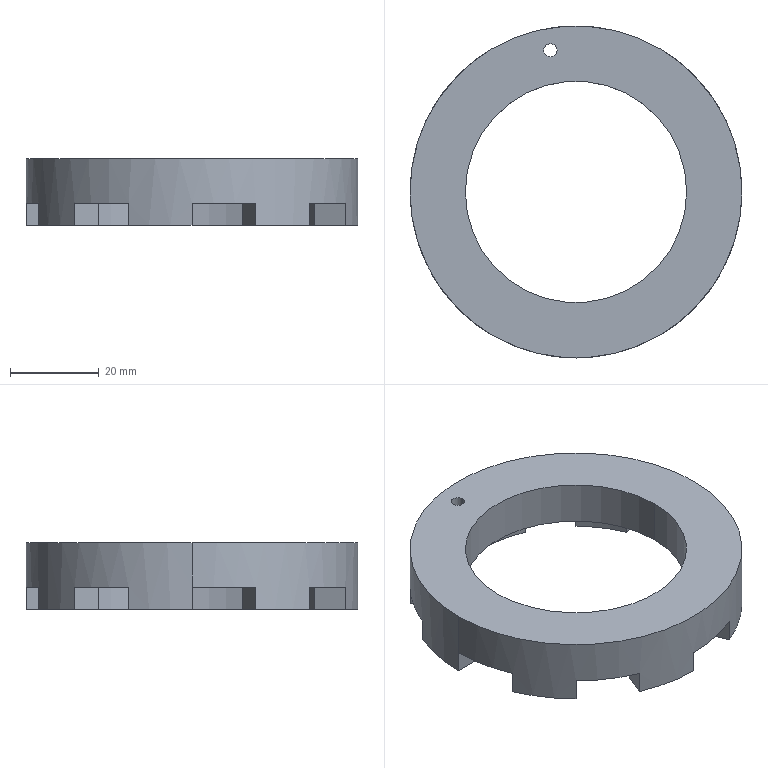Part | SolidWorks | features ICE 3, Extrusion 1 | 1 solid | 40 faces | box 75 x 75 x 15 mm | volume 28449 mm3 | plane 26 | cylinder 14 | commonest cylinder face diameters 60 x8 3 x2 50 x2 75 x2
STEP:
#1=CARTESIAN_POINT('',(-4.276,31.983,15.));
#2=VERTEX_POINT('',#1);
#3=CARTESIAN_POINT('',(-7.276,31.983,15.));
#4=VERTEX_POINT('',#3);
#5=CARTESIAN_POINT('',(-5.776,31.983,15.));
#6=DIRECTION('',(0.,0.,-1.));
#7=DIRECTION('',(-1.,0.,0.));
#8=AXIS2_PLACEMENT_3D('',#5,#6,#7);
#9=CIRCLE('',#8,1.5);
#10=EDGE_CURVE('',#2,#4,#9,.T.);
#11=ORIENTED_EDGE('',*,*,#10,.F.);
#12=CARTESIAN_POINT('',(-4.276,31.983,5.));
#13=VERTEX_POINT('',#12);
#14=CARTESIAN_POINT('',(-4.276,31.983,15.));
#15=DIRECTION('',(0.,0.,-1.));
#16=VECTOR('',#15,1000.);
#17=LINE('',#14,#16);
#18=EDGE_CURVE('',#2,#13,#17,.T.);
#19=ORIENTED_EDGE('',*,*,#18,.T.);
#20=CARTESIAN_POINT('',(-7.276,31.983,5.));
#21=VERTEX_POINT('',#20);
#22=CARTESIAN_POINT('',(-5.776,31.983,5.));
#23=DIRECTION('',(0.,0.,-1.));
#24=DIRECTION('',(-1.,0.,0.));
#25=AXIS2_PLACEMENT_3D('',#22,#23,#24);
#26=CIRCLE('',#25,1.5);
#27=EDGE_CURVE('',#13,#21,#26,.T.);
#28=ORIENTED_EDGE('',*,*,#27,.T.);
#29=CARTESIAN_POINT('',(-7.276,31.983,15.));
#30=DIRECTION('',(0.,0.,-1.));
#31=VECTOR('',#30,1000.);
#32=LINE('',#29,#31);
#33=EDGE_CURVE('',#4,#21,#32,.T.);
#34=ORIENTED_EDGE('',*,*,#33,.F.);
#35=EDGE_LOOP('',(#11,#19,#28,#34));
#36=FACE_OUTER_BOUND('',#35,.T.);
#37=CARTESIAN_POINT('',(-5.776,31.983,15.));
#38=DIRECTION('',(0.,0.,-1.));
#39=DIRECTION('',(-1.,0.,0.));
#40=AXIS2_PLACEMENT_3D('',#37,#38,#39);
#41=CYLINDRICAL_SURFACE('',#40,1.5);
#42=ADVANCED_FACE('',(#36),#41,.F.);
#43=CARTESIAN_POINT('',(37.5,0.,15.));
#44=VERTEX_POINT('',#43);
#45=CARTESIAN_POINT('',(-37.5,0.,15.));
#46=VERTEX_POINT('',#45);
#47=CARTESIAN_POINT('',(0.,0.,15.));
#48=DIRECTION('',(0.,0.,1.));
#49=DIRECTION('',(1.,0.,0.));
#50=AXIS2_PLACEMENT_3D('',#47,#48,#49);
#51=CIRCLE('',#50,37.5);
#52=EDGE_CURVE('',#44,#46,#51,.T.);
#53=ORIENTED_EDGE('',*,*,#52,.F.);
#54=CARTESIAN_POINT('',(37.5,0.,5.));
#55=VERTEX_POINT('',#54);
#56=CARTESIAN_POINT('',(37.5,0.,15.));
#57=DIRECTION('',(0.,0.,-1.));
#58=VECTOR('',#57,1000.);
#59=LINE('',#56,#58);
#60=EDGE_CURVE('',#44,#55,#59,.T.);
#61=ORIENTED_EDGE('',*,*,#60,.T.);
#62=CARTESIAN_POINT('',(34.645,14.351,5.));
#63=VERTEX_POINT('',#62);
#64=CARTESIAN_POINT('',(0.,0.,5.));
#65=DIRECTION('',(0.,0.,-1.));
#66=DIRECTION('',(-1.,0.,0.));
#67=AXIS2_PLACEMENT_3D('',#64,#65,#66);
#68=CIRCLE('',#67,37.5);
#69=EDGE_CURVE('',#63,#55,#68,.T.);
#70=ORIENTED_EDGE('',*,*,#69,.F.);
#71=CARTESIAN_POINT('',(34.645,14.351,0.));
#72=VERTEX_POINT('',#71);
#73=CARTESIAN_POINT('',(34.645,14.351,5.));
#74=DIRECTION('',(0.,0.,-1.));
#75=VECTOR('',#74,1000.);
#76=LINE('',#73,#75);
#77=EDGE_CURVE('',#63,#72,#76,.T.);
#78=ORIENTED_EDGE('',*,*,#77,.T.);
#79=CARTESIAN_POINT('',(26.517,26.517,0.));
#80=VERTEX_POINT('',#79);
#81=CARTESIAN_POINT('',(0.,0.,0.));
#82=DIRECTION('',(0.,0.,1.));
#83=DIRECTION('',(1.,0.,0.));
#84=AXIS2_PLACEMENT_3D('',#81,#82,#83);
#85=CIRCLE('',#84,37.5);
#86=EDGE_CURVE('',#72,#80,#85,.T.);
#87=ORIENTED_EDGE('',*,*,#86,.T.);
#88=CARTESIAN_POINT('',(26.517,26.517,5.));
#89=VERTEX_POINT('',#88);
#90=CARTESIAN_POINT('',(26.517,26.517,5.));
#91=DIRECTION('',(0.,0.,-1.));
#92=VECTOR('',#91,1000.);
#93=LINE('',#90,#92);
#94=EDGE_CURVE('',#89,#80,#93,.T.);
#95=ORIENTED_EDGE('',*,*,#94,.F.);
#96=CARTESIAN_POINT('',(14.351,34.645,5.));
#97=VERTEX_POINT('',#96);
#98=CARTESIAN_POINT('',(0.,0.,5.));
#99=DIRECTION('',(0.,0.,-1.));
#100=DIRECTION('',(-1.,0.,0.));
#101=AXIS2_PLACEMENT_3D('',#98,#99,#100);
#102=CIRCLE('',#101,37.5);
#103=EDGE_CURVE('',#97,#89,#102,.T.);
#104=ORIENTED_EDGE('',*,*,#103,.F.);
#105=CARTESIAN_POINT('',(14.351,34.645,0.));
#106=VERTEX_POINT('',#105);
#107=CARTESIAN_POINT('',(14.351,34.645,5.));
#108=DIRECTION('',(0.,0.,-1.));
#109=VECTOR('',#108,1000.);
#110=LINE('',#107,#109);
#111=EDGE_CURVE('',#97,#106,#110,.T.);
#112=ORIENTED_EDGE('',*,*,#111,.T.);
#113=CARTESIAN_POINT('',(0.,37.5,0.));
#114=VERTEX_POINT('',#113);
#115=CARTESIAN_POINT('',(0.,0.,0.));
#116=DIRECTION('',(0.,0.,1.));
#117=DIRECTION('',(1.,0.,0.));
#118=AXIS2_PLACEMENT_3D('',#115,#116,#117);
#119=CIRCLE('',#118,37.5);
#120=EDGE_CURVE('',#106,#114,#119,.T.);
#121=ORIENTED_EDGE('',*,*,#120,.T.);
#122=CARTESIAN_POINT('',(0.,37.5,5.));
#123=VERTEX_POINT('',#122);
#124=CARTESIAN_POINT('',(0.,37.5,5.));
#125=DIRECTION('',(0.,0.,-1.));
#126=VECTOR('',#125,1000.);
#127=LINE('',#124,#126);
#128=EDGE_CURVE('',#123,#114,#127,.T.);
#129=ORIENTED_EDGE('',*,*,#128,.F.);
#130=CARTESIAN_POINT('',(-14.351,34.645,5.));
#131=VERTEX_POINT('',#130);
#132=CARTESIAN_POINT('',(0.,0.,5.));
#133=DIRECTION('',(0.,0.,-1.));
#134=DIRECTION('',(-1.,0.,0.));
#135=AXIS2_PLACEMENT_3D('',#132,#133,#134);
#136=CIRCLE('',#135,37.5);
#137=EDGE_CURVE('',#131,#123,#136,.T.);
#138=ORIENTED_EDGE('',*,*,#137,.F.);
#139=CARTESIAN_POINT('',(-14.351,34.645,0.));
#140=VERTEX_POINT('',#139);
#141=CARTESIAN_POINT('',(-14.351,34.645,5.));
#142=DIRECTION('',(0.,0.,-1.));
#143=VECTOR('',#142,1000.);
#144=LINE('',#141,#143);
#145=EDGE_CURVE('',#131,#140,#144,.T.);
#146=ORIENTED_EDGE('',*,*,#145,.T.);
#147=CARTESIAN_POINT('',(-26.517,26.517,0.));
#148=VERTEX_POINT('',#147);
#149=CARTESIAN_POINT('',(0.,0.,0.));
#150=DIRECTION('',(0.,0.,1.));
#151=DIRECTION('',(1.,0.,0.));
#152=AXIS2_PLACEMENT_3D('',#149,#150,#151);
#153=CIRCLE('',#152,37.5);
#154=EDGE_CURVE('',#140,#148,#153,.T.);
#155=ORIENTED_EDGE('',*,*,#154,.T.);
#156=CARTESIAN_POINT('',(-26.517,26.517,5.));
#157=VERTEX_POINT('',#156);
#158=CARTESIAN_POINT('',(-26.517,26.517,5.));
#159=DIRECTION('',(0.,0.,-1.));
#160=VECTOR('',#159,1000.);
#161=LINE('',#158,#160);
#162=EDGE_CURVE('',#157,#148,#161,.T.);
#163=ORIENTED_EDGE('',*,*,#162,.F.);
#164=CARTESIAN_POINT('',(-34.645,14.351,5.));
#165=VERTEX_POINT('',#164);
#166=CARTESIAN_POINT('',(0.,0.,5.));
#167=DIRECTION('',(0.,0.,-1.));
#168=DIRECTION('',(-1.,0.,0.));
#169=AXIS2_PLACEMENT_3D('',#166,#167,#168);
#170=CIRCLE('',#169,37.5);
#171=EDGE_CURVE('',#165,#157,#170,.T.);
#172=ORIENTED_EDGE('',*,*,#171,.F.);
#173=CARTESIAN_POINT('',(-34.645,14.351,0.));
#174=VERTEX_POINT('',#173);
#175=CARTESIAN_POINT('',(-34.645,14.351,5.));
#176=DIRECTION('',(0.,0.,-1.));
#177=VECTOR('',#176,1000.);
#178=LINE('',#175,#177);
#179=EDGE_CURVE('',#165,#174,#178,.T.);
#180=ORIENTED_EDGE('',*,*,#179,.T.);
#181=CARTESIAN_POINT('',(-37.5,0.,0.));
#182=VERTEX_POINT('',#181);
#183=CARTESIAN_POINT('',(0.,0.,0.));
#184=DIRECTION('',(0.,0.,1.));
#185=DIRECTION('',(1.,0.,0.));
#186=AXIS2_PLACEMENT_3D('',#183,#184,#185);
#187=CIRCLE('',#186,37.5);
#188=EDGE_CURVE('',#174,#182,#187,.T.);
#189=ORIENTED_EDGE('',*,*,#188,.T.);
#190=CARTESIAN_POINT('',(-37.5,0.,5.));
#191=VERTEX_POINT('',#190);
#192=CARTESIAN_POINT('',(-37.5,0.,5.));
#193=DIRECTION('',(0.,0.,-1.));
#194=VECTOR('',#193,1000.);
#195=LINE('',#192,#194);
#196=EDGE_CURVE('',#191,#182,#195,.T.);
#197=ORIENTED_EDGE('',*,*,#196,.F.);
#198=CARTESIAN_POINT('',(-37.5,0.,15.));
#199=DIRECTION('',(0.,0.,-1.));
#200=VECTOR('',#199,1000.);
#201=LINE('',#198,#200);
#202=EDGE_CURVE('',#46,#191,#201,.T.);
#203=ORIENTED_EDGE('',*,*,#202,.F.);
#204=EDGE_LOOP('',(#53,#61,#70,#78,#87,#95,#104,#112,#121,#129,#138,#146,#155,#163,#172,#180,#189,#197,#203));
#205=FACE_OUTER_BOUND('',#204,.T.);
#206=CARTESIAN_POINT('',(0.,0.,15.));
#207=DIRECTION('',(0.,0.,-1.));
#208=DIRECTION('',(-1.,0.,0.));
#209=AXIS2_PLACEMENT_3D('',#206,#207,#208);
#210=CYLINDRICAL_SURFACE('',#209,37.5);
#211=ADVANCED_FACE('',(#205),#210,.T.);
#212=CARTESIAN_POINT('',(-25.,0.,15.));
#213=VERTEX_POINT('',#212);
#214=CARTESIAN_POINT('',(25.,0.,15.));
#215=VERTEX_POINT('',#214);
#216=CARTESIAN_POINT('',(0.,0.,15.));
#217=DIRECTION('',(0.,0.,1.));
#218=DIRECTION('',(1.,0.,0.));
#219=AXIS2_PLACEMENT_3D('',#216,#217,#218);
#220=CIRCLE('',#219,25.);
#221=EDGE_CURVE('',#213,#215,#220,.T.);
#222=ORIENTED_EDGE('',*,*,#221,.T.);
#223=CARTESIAN_POINT('',(25.,0.,5.));
#224=VERTEX_POINT('',#223);
#225=CARTESIAN_POINT('',(25.,0.,15.));
#226=DIRECTION('',(0.,0.,-1.));
#227=VECTOR('',#226,1000.);
#228=LINE('',#225,#227);
#229=EDGE_CURVE('',#215,#224,#228,.T.);
#230=ORIENTED_EDGE('',*,*,#229,.T.);
#231=CARTESIAN_POINT('',(-25.,0.,5.));
#232=VERTEX_POINT('',#231);
#233=CARTESIAN_POINT('',(0.,0.,5.));
#234=DIRECTION('',(0.,0.,-1.));
#235=DIRECTION('',(-1.,0.,0.));
#236=AXIS2_PLACEMENT_3D('',#233,#234,#235);
#237=CIRCLE('',#236,25.);
#238=EDGE_CURVE('',#224,#232,#237,.T.);
#239=ORIENTED_EDGE('',*,*,#238,.T.);
#240=CARTESIAN_POINT('',(-25.,0.,15.));
#241=DIRECTION('',(0.,0.,-1.));
#242=VECTOR('',#241,1000.);
#243=LINE('',#240,#242);
#244=EDGE_CURVE('',#213,#232,#243,.T.);
#245=ORIENTED_EDGE('',*,*,#244,.F.);
#246=EDGE_LOOP('',(#222,#230,#239,#245));
#247=FACE_OUTER_BOUND('',#246,.T.);
#248=CARTESIAN_POINT('',(0.,0.,15.));
#249=DIRECTION('',(0.,0.,-1.));
#250=DIRECTION('',(-1.,0.,0.));
#251=AXIS2_PLACEMENT_3D('',#248,#249,#250);
#252=CYLINDRICAL_SURFACE('',#251,25.);
#253=ADVANCED_FACE('',(#247),#252,.F.);
#254=CARTESIAN_POINT('',(-14.351,-34.645,0.));
#255=VERTEX_POINT('',#254);
#256=CARTESIAN_POINT('',(0.,-37.5,0.));
#257=VERTEX_POINT('',#256);
#258=CARTESIAN_POINT('',(0.,0.,0.));
#259=DIRECTION('',(0.,0.,1.));
#260=DIRECTION('',(1.,0.,0.));
#261=AXIS2_PLACEMENT_3D('',#258,#259,#260);
#262=CIRCLE('',#261,37.5);
#263=EDGE_CURVE('',#255,#257,#262,.T.);
#264=ORIENTED_EDGE('',*,*,#263,.F.);
#265=CARTESIAN_POINT('',(-11.481,-27.716,0.));
#266=VERTEX_POINT('',#265);
#267=CARTESIAN_POINT('',(-11.481,-27.716,0.));
#268=DIRECTION('',(-0.3827,-0.9239,0.));
#269=VECTOR('',#268,1000.);
#270=LINE('',#267,#269);
#271=EDGE_CURVE('',#266,#255,#270,.T.);
#272=ORIENTED_EDGE('',*,*,#271,.F.);
#273=CARTESIAN_POINT('',(0.,-30.,0.));
#274=VERTEX_POINT('',#273);
#275=CARTESIAN_POINT('',(0.,0.,0.));
#276=DIRECTION('',(0.,0.,-1.));
#277=DIRECTION('',(-1.,0.,0.));
#278=AXIS2_PLACEMENT_3D('',#275,#276,#277);
#279=CIRCLE('',#278,30.);
#280=EDGE_CURVE('',#274,#266,#279,.T.);
#281=ORIENTED_EDGE('',*,*,#280,.F.);
#282=CARTESIAN_POINT('',(0.,-30.,0.));
#283=DIRECTION('',(0.,1.,0.));
#284=VECTOR('',#283,1000.);
#285=LINE('',#282,#284);
#286=EDGE_CURVE('',#257,#274,#285,.T.);
#287=ORIENTED_EDGE('',*,*,#286,.F.);
#288=EDGE_LOOP('',(#264,#272,#281,#287));
#289=FACE_OUTER_BOUND('',#288,.T.);
#290=CARTESIAN_POINT('',(0.,0.,0.));
#291=DIRECTION('',(0.,0.,1.));
#292=DIRECTION('',(1.,0.,0.));
#293=AXIS2_PLACEMENT_3D('',#290,#291,#292);
#294=PLANE('',#293);
#295=ADVANCED_FACE('',(#289),#294,.F.);
#296=CARTESIAN_POINT('',(-21.213,21.213,0.));
#297=VERTEX_POINT('',#296);
#298=CARTESIAN_POINT('',(-11.481,27.716,0.));
#299=VERTEX_POINT('',#298);
#300=CARTESIAN_POINT('',(0.,0.,0.));
#301=DIRECTION('',(0.,0.,-1.));
#302=DIRECTION('',(-1.,0.,0.));
#303=AXIS2_PLACEMENT_3D('',#300,#301,#302);
#304=CIRCLE('',#303,30.);
#305=EDGE_CURVE('',#297,#299,#304,.T.);
#306=ORIENTED_EDGE('',*,*,#305,.F.);
#307=CARTESIAN_POINT('',(-21.213,21.213,0.));
#308=DIRECTION('',(0.7071,-0.7071,0.));
#309=VECTOR('',#308,1000.);
#310=LINE('',#307,#309);
#311=EDGE_CURVE('',#148,#297,#310,.T.);
#312=ORIENTED_EDGE('',*,*,#311,.F.);
#313=ORIENTED_EDGE('',*,*,#154,.F.);
#314=CARTESIAN_POINT('',(-11.481,27.716,0.));
#315=DIRECTION('',(-0.3827,0.9239,0.));
#316=VECTOR('',#315,1000.);
#317=LINE('',#314,#316);
#318=EDGE_CURVE('',#299,#140,#317,.T.);
#319=ORIENTED_EDGE('',*,*,#318,.F.);
#320=EDGE_LOOP('',(#306,#312,#313,#319));
#321=FACE_OUTER_BOUND('',#320,.T.);
#322=CARTESIAN_POINT('',(0.,0.,0.));
#323=DIRECTION('',(0.,0.,1.));
#324=DIRECTION('',(1.,0.,0.));
#325=AXIS2_PLACEMENT_3D('',#322,#323,#324);
#326=PLANE('',#325);
#327=ADVANCED_FACE('',(#321),#326,.F.);
#328=ORIENTED_EDGE('',*,*,#188,.F.);
#329=CARTESIAN_POINT('',(-27.716,11.481,0.));
#330=VERTEX_POINT('',#329);
#331=CARTESIAN_POINT('',(-27.716,11.481,0.));
#332=DIRECTION('',(-0.9239,0.3827,0.));
#333=VECTOR('',#332,1000.);
#334=LINE('',#331,#333);
#335=EDGE_CURVE('',#330,#174,#334,.T.);
#336=ORIENTED_EDGE('',*,*,#335,.F.);
#337=CARTESIAN_POINT('',(-30.,0.,0.));
#338=VERTEX_POINT('',#337);
#339=CARTESIAN_POINT('',(0.,0.,0.));
#340=DIRECTION('',(0.,0.,-1.));
#341=DIRECTION('',(-1.,0.,0.));
#342=AXIS2_PLACEMENT_3D('',#339,#340,#341);
#343=CIRCLE('',#342,30.);
#344=EDGE_CURVE('',#338,#330,#343,.T.);
#345=ORIENTED_EDGE('',*,*,#344,.F.);
#346=CARTESIAN_POINT('',(-30.,0.,0.));
#347=DIRECTION('',(1.,0.,0.));
#348=VECTOR('',#347,1000.);
#349=LINE('',#346,#348);
#350=EDGE_CURVE('',#182,#338,#349,.T.);
#351=ORIENTED_EDGE('',*,*,#350,.F.);
#352=EDGE_LOOP('',(#328,#336,#345,#351));
#353=FACE_OUTER_BOUND('',#352,.T.);
#354=CARTESIAN_POINT('',(0.,0.,0.));
#355=DIRECTION('',(0.,0.,1.));
#356=DIRECTION('',(1.,0.,0.));
#357=AXIS2_PLACEMENT_3D('',#354,#355,#356);
#358=PLANE('',#357);
#359=ADVANCED_FACE('',(#353),#358,.F.);
#360=CARTESIAN_POINT('',(14.351,-34.645,0.));
#361=VERTEX_POINT('',#360);
#362=CARTESIAN_POINT('',(26.517,-26.517,0.));
#363=VERTEX_POINT('',#362);
#364=CARTESIAN_POINT('',(0.,0.,0.));
#365=DIRECTION('',(0.,0.,1.));
#366=DIRECTION('',(1.,0.,0.));
#367=AXIS2_PLACEMENT_3D('',#364,#365,#366);
#368=CIRCLE('',#367,37.5);
#369=EDGE_CURVE('',#361,#363,#368,.T.);
#370=ORIENTED_EDGE('',*,*,#369,.F.);
#371=CARTESIAN_POINT('',(11.481,-27.716,0.));
#372=VERTEX_POINT('',#371);
#373=CARTESIAN_POINT('',(11.481,-27.716,0.));
#374=DIRECTION('',(0.3827,-0.9239,0.));
#375=VECTOR('',#374,1000.);
#376=LINE('',#373,#375);
#377=EDGE_CURVE('',#372,#361,#376,.T.);
#378=ORIENTED_EDGE('',*,*,#377,.F.);
#379=CARTESIAN_POINT('',(21.213,-21.213,0.));
#380=VERTEX_POINT('',#379);
#381=CARTESIAN_POINT('',(0.,0.,0.));
#382=DIRECTION('',(0.,0.,-1.));
#383=DIRECTION('',(-1.,0.,0.));
#384=AXIS2_PLACEMENT_3D('',#381,#382,#383);
#385=CIRCLE('',#384,30.);
#386=EDGE_CURVE('',#380,#372,#385,.T.);
#387=ORIENTED_EDGE('',*,*,#386,.F.);
#388=CARTESIAN_POINT('',(21.213,-21.213,0.));
#389=DIRECTION('',(-0.7071,0.7071,0.));
#390=VECTOR('',#389,1000.);
#391=LINE('',#388,#390);
#392=EDGE_CURVE('',#363,#380,#391,.T.);
#393=ORIENTED_EDGE('',*,*,#392,.F.);
#394=EDGE_LOOP('',(#370,#378,#387,#393));
#395=FACE_OUTER_BOUND('',#394,.T.);
#396=CARTESIAN_POINT('',(0.,0.,0.));
#397=DIRECTION('',(0.,0.,1.));
#398=DIRECTION('',(1.,0.,0.));
#399=AXIS2_PLACEMENT_3D('',#396,#397,#398);
#400=PLANE('',#399);
#401=ADVANCED_FACE('',(#395),#400,.F.);
#402=CARTESIAN_POINT('',(34.645,-14.351,0.));
#403=VERTEX_POINT('',#402);
#404=CARTESIAN_POINT('',(37.5,0.,0.));
#405=VERTEX_POINT('',#404);
#406=CARTESIAN_POINT('',(0.,0.,0.));
#407=DIRECTION('',(0.,0.,1.));
#408=DIRECTION('',(1.,0.,0.));
#409=AXIS2_PLACEMENT_3D('',#406,#407,#408);
#410=CIRCLE('',#409,37.5);
#411=EDGE_CURVE('',#403,#405,#410,.T.);
#412=ORIENTED_EDGE('',*,*,#411,.F.);
#413=CARTESIAN_POINT('',(27.716,-11.481,0.));
#414=VERTEX_POINT('',#413);
#415=CARTESIAN_POINT('',(27.716,-11.481,0.));
#416=DIRECTION('',(0.9239,-0.3827,0.));
#417=VECTOR('',#416,1000.);
#418=LINE('',#415,#417);
#419=EDGE_CURVE('',#414,#403,#418,.T.);
#420=ORIENTED_EDGE('',*,*,#419,.F.);
#421=CARTESIAN_POINT('',(30.,0.,0.));
#422=VERTEX_POINT('',#421);
#423=CARTESIAN_POINT('',(0.,0.,0.));
#424=DIRECTION('',(0.,0.,-1.));
#425=DIRECTION('',(-1.,0.,0.));
#426=AXIS2_PLACEMENT_3D('',#423,#424,#425);
#427=CIRCLE('',#426,30.);
#428=EDGE_CURVE('',#422,#414,#427,.T.);
#429=ORIENTED_EDGE('',*,*,#428,.F.);
#430=CARTESIAN_POINT('',(30.,0.,0.));
#431=DIRECTION('',(-1.,0.,0.));
#432=VECTOR('',#431,1000.);
#433=LINE('',#430,#432);
#434=EDGE_CURVE('',#405,#422,#433,.T.);
#435=ORIENTED_EDGE('',*,*,#434,.F.);
#436=EDGE_LOOP('',(#412,#420,#429,#435));
#437=FACE_OUTER_BOUND('',#436,.T.);
#438=CARTESIAN_POINT('',(0.,0.,0.));
#439=DIRECTION('',(0.,0.,1.));
#440=DIRECTION('',(1.,0.,0.));
#441=AXIS2_PLACEMENT_3D('',#438,#439,#440);
#442=PLANE('',#441);
#443=ADVANCED_FACE('',(#437),#442,.F.);
#444=ORIENTED_EDGE('',*,*,#86,.F.);
#445=CARTESIAN_POINT('',(27.716,11.481,0.));
#446=VERTEX_POINT('',#445);
#447=CARTESIAN_POINT('',(27.716,11.481,0.));
#448=DIRECTION('',(0.9239,0.3827,0.));
#449=VECTOR('',#448,1000.);
#450=LINE('',#447,#449);
#451=EDGE_CURVE('',#446,#72,#450,.T.);
#452=ORIENTED_EDGE('',*,*,#451,.F.);
#453=CARTESIAN_POINT('',(21.213,21.213,0.));
#454=VERTEX_POINT('',#453);
#455=CARTESIAN_POINT('',(0.,0.,0.));
#456=DIRECTION('',(0.,0.,-1.));
#457=DIRECTION('',(-1.,0.,0.));
#458=AXIS2_PLACEMENT_3D('',#455,#456,#457);
#459=CIRCLE('',#458,30.);
#460=EDGE_CURVE('',#454,#446,#459,.T.);
#461=ORIENTED_EDGE('',*,*,#460,.F.);
#462=CARTESIAN_POINT('',(21.213,21.213,0.));
#463=DIRECTION('',(-0.7071,-0.7071,0.));
#464=VECTOR('',#463,1000.);
#465=LINE('',#462,#464);
#466=EDGE_CURVE('',#80,#454,#465,.T.);
#467=ORIENTED_EDGE('',*,*,#466,.F.);
#468=EDGE_LOOP('',(#444,#452,#461,#467));
#469=FACE_OUTER_BOUND('',#468,.T.);
#470=CARTESIAN_POINT('',(0.,0.,0.));
#471=DIRECTION('',(0.,0.,1.));
#472=DIRECTION('',(1.,0.,0.));
#473=AXIS2_PLACEMENT_3D('',#470,#471,#472);
#474=PLANE('',#473);
#475=ADVANCED_FACE('',(#469),#474,.F.);
#476=ORIENTED_EDGE('',*,*,#120,.F.);
#477=CARTESIAN_POINT('',(11.481,27.716,0.));
#478=VERTEX_POINT('',#477);
#479=CARTESIAN_POINT('',(11.481,27.716,0.));
#480=DIRECTION('',(0.3827,0.9239,0.));
#481=VECTOR('',#480,1000.);
#482=LINE('',#479,#481);
#483=EDGE_CURVE('',#478,#106,#482,.T.);
#484=ORIENTED_EDGE('',*,*,#483,.F.);
#485=CARTESIAN_POINT('',(0.,30.,0.));
#486=VERTEX_POINT('',#485);
#487=CARTESIAN_POINT('',(0.,0.,0.));
#488=DIRECTION('',(0.,0.,-1.));
#489=DIRECTION('',(-1.,0.,0.));
#490=AXIS2_PLACEMENT_3D('',#487,#488,#489);
#491=CIRCLE('',#490,30.);
#492=EDGE_CURVE('',#486,#478,#491,.T.);
#493=ORIENTED_EDGE('',*,*,#492,.F.);
#494=CARTESIAN_POINT('',(0.,30.,0.));
#495=DIRECTION('',(0.,-1.,0.));
#496=VECTOR('',#495,1000.);
#497=LINE('',#494,#496);
#498=EDGE_CURVE('',#114,#486,#497,.T.);
#499=ORIENTED_EDGE('',*,*,#498,.F.);
#500=EDGE_LOOP('',(#476,#484,#493,#499));
#501=FACE_OUTER_BOUND('',#500,.T.);
#502=CARTESIAN_POINT('',(0.,0.,0.));
#503=DIRECTION('',(0.,0.,1.));
#504=DIRECTION('',(1.,0.,0.));
#505=AXIS2_PLACEMENT_3D('',#502,#503,#504);
#506=PLANE('',#505);
#507=ADVANCED_FACE('',(#501),#506,.F.);
#508=ORIENTED_EDGE('',*,*,#280,.T.);
#509=CARTESIAN_POINT('',(-11.481,-27.716,5.));
#510=VERTEX_POINT('',#509);
#511=CARTESIAN_POINT('',(-11.481,-27.716,5.));
#512=DIRECTION('',(0.,0.,-1.));
#513=VECTOR('',#512,1000.);
#514=LINE('',#511,#513);
#515=EDGE_CURVE('',#510,#266,#514,.T.);
#516=ORIENTED_EDGE('',*,*,#515,.F.);
#517=CARTESIAN_POINT('',(0.,-30.,5.));
#518=VERTEX_POINT('',#517);
#519=CARTESIAN_POINT('',(0.,0.,5.));
#520=DIRECTION('',(0.,0.,-1.));
#521=DIRECTION('',(-1.,0.,0.));
#522=AXIS2_PLACEMENT_3D('',#519,#520,#521);
#523=CIRCLE('',#522,30.);
#524=EDGE_CURVE('',#518,#510,#523,.T.);
#525=ORIENTED_EDGE('',*,*,#524,.F.);
#526=CARTESIAN_POINT('',(0.,-30.,5.));
#527=DIRECTION('',(0.,0.,-1.));
#528=VECTOR('',#527,1000.);
#529=LINE('',#526,#528);
#530=EDGE_CURVE('',#518,#274,#529,.T.);
#531=ORIENTED_EDGE('',*,*,#530,.T.);
#532=EDGE_LOOP('',(#508,#516,#525,#531));
#533=FACE_OUTER_BOUND('',#532,.T.);
#534=CARTESIAN_POINT('',(0.,0.,5.));
#535=DIRECTION('',(0.,0.,-1.));
#536=DIRECTION('',(-1.,0.,0.));
#537=AXIS2_PLACEMENT_3D('',#534,#535,#536);
#538=CYLINDRICAL_SURFACE('',#537,30.);
#539=ADVANCED_FACE('',(#533),#538,.F.);
#540=CARTESIAN_POINT('',(-21.213,21.213,5.));
#541=VERTEX_POINT('',#540);
#542=CARTESIAN_POINT('',(-11.481,27.716,5.));
#543=VERTEX_POINT('',#542);
#544=CARTESIAN_POINT('',(0.,0.,5.));
#545=DIRECTION('',(0.,0.,-1.));
#546=DIRECTION('',(-1.,0.,0.));
#547=AXIS2_PLACEMENT_3D('',#544,#545,#546);
#548=CIRCLE('',#547,30.);
#549=EDGE_CURVE('',#541,#543,#548,.T.);
#550=ORIENTED_EDGE('',*,*,#549,.F.);
#551=CARTESIAN_POINT('',(-21.213,21.213,5.));
#552=DIRECTION('',(0.,0.,-1.));
#553=VECTOR('',#552,1000.);
#554=LINE('',#551,#553);
#555=EDGE_CURVE('',#541,#297,#554,.T.);
#556=ORIENTED_EDGE('',*,*,#555,.T.);
#557=ORIENTED_EDGE('',*,*,#305,.T.);
#558=CARTESIAN_POINT('',(-11.481,27.716,5.));
#559=DIRECTION('',(0.,0.,-1.));
#560=VECTOR('',#559,1000.);
#561=LINE('',#558,#560);
#562=EDGE_CURVE('',#543,#299,#561,.T.);
#563=ORIENTED_EDGE('',*,*,#562,.F.);
#564=EDGE_LOOP('',(#550,#556,#557,#563));
#565=FACE_OUTER_BOUND('',#564,.T.);
#566=CARTESIAN_POINT('',(0.,0.,5.));
#567=DIRECTION('',(0.,0.,-1.));
#568=DIRECTION('',(-1.,0.,0.));
#569=AXIS2_PLACEMENT_3D('',#566,#567,#568);
#570=CYLINDRICAL_SURFACE('',#569,30.);
#571=ADVANCED_FACE('',(#565),#570,.F.);
#572=ORIENTED_EDGE('',*,*,#344,.T.);
#573=CARTESIAN_POINT('',(-27.716,11.481,5.));
#574=VERTEX_POINT('',#573);
#575=CARTESIAN_POINT('',(-27.716,11.481,5.));
#576=DIRECTION('',(0.,0.,-1.));
#577=VECTOR('',#576,1000.);
#578=LINE('',#575,#577);
#579=EDGE_CURVE('',#574,#330,#578,.T.);
#580=ORIENTED_EDGE('',*,*,#579,.F.);
#581=CARTESIAN_POINT('',(-30.,0.,5.));
#582=VERTEX_POINT('',#581);
#583=CARTESIAN_POINT('',(0.,0.,5.));
#584=DIRECTION('',(0.,0.,-1.));
#585=DIRECTION('',(-1.,0.,0.));
#586=AXIS2_PLACEMENT_3D('',#583,#584,#585);
#587=CIRCLE('',#586,30.);
#588=EDGE_CURVE('',#582,#574,#587,.T.);
#589=ORIENTED_EDGE('',*,*,#588,.F.);
#590=CARTESIAN_POINT('',(-30.,0.,5.));
#591=DIRECTION('',(0.,0.,-1.));
#592=VECTOR('',#591,1000.);
#593=LINE('',#590,#592);
#594=EDGE_CURVE('',#582,#338,#593,.T.);
#595=ORIENTED_EDGE('',*,*,#594,.T.);
#596=EDGE_LOOP('',(#572,#580,#589,#595));
#597=FACE_OUTER_BOUND('',#596,.T.);
#598=CARTESIAN_POINT('',(0.,0.,5.));
#599=DIRECTION('',(0.,0.,-1.));
#600=DIRECTION('',(-1.,0.,0.));
#601=AXIS2_PLACEMENT_3D('',#598,#599,#600);
#602=CYLINDRICAL_SURFACE('',#601,30.);
#603=ADVANCED_FACE('',(#597),#602,.F.);
#604=ORIENTED_EDGE('',*,*,#386,.T.);
#605=CARTESIAN_POINT('',(11.481,-27.716,5.));
#606=VERTEX_POINT('',#605);
#607=CARTESIAN_POINT('',(11.481,-27.716,5.));
#608=DIRECTION('',(0.,0.,-1.));
#609=VECTOR('',#608,1000.);
#610=LINE('',#607,#609);
#611=EDGE_CURVE('',#606,#372,#610,.T.);
#612=ORIENTED_EDGE('',*,*,#611,.F.);
#613=CARTESIAN_POINT('',(21.213,-21.213,5.));
#614=VERTEX_POINT('',#613);
#615=CARTESIAN_POINT('',(0.,0.,5.));
#616=DIRECTION('',(0.,0.,-1.));
#617=DIRECTION('',(-1.,0.,0.));
#618=AXIS2_PLACEMENT_3D('',#615,#616,#617);
#619=CIRCLE('',#618,30.);
#620=EDGE_CURVE('',#614,#606,#619,.T.);
#621=ORIENTED_EDGE('',*,*,#620,.F.);
#622=CARTESIAN_POINT('',(21.213,-21.213,5.));
#623=DIRECTION('',(0.,0.,-1.));
#624=VECTOR('',#623,1000.);
#625=LINE('',#622,#624);
#626=EDGE_CURVE('',#614,#380,#625,.T.);
#627=ORIENTED_EDGE('',*,*,#626,.T.);
#628=EDGE_LOOP('',(#604,#612,#621,#627));
#629=FACE_OUTER_BOUND('',#628,.T.);
#630=CARTESIAN_POINT('',(0.,0.,5.));
#631=DIRECTION('',(0.,0.,-1.));
#632=DIRECTION('',(-1.,0.,0.));
#633=AXIS2_PLACEMENT_3D('',#630,#631,#632);
#634=CYLINDRICAL_SURFACE('',#633,30.);
#635=ADVANCED_FACE('',(#629),#634,.F.);
#636=ORIENTED_EDGE('',*,*,#428,.T.);
#637=CARTESIAN_POINT('',(27.716,-11.481,5.));
#638=VERTEX_POINT('',#637);
#639=CARTESIAN_POINT('',(27.716,-11.481,5.));
#640=DIRECTION('',(0.,0.,-1.));
#641=VECTOR('',#640,1000.);
#642=LINE('',#639,#641);
#643=EDGE_CURVE('',#638,#414,#642,.T.);
#644=ORIENTED_EDGE('',*,*,#643,.F.);
#645=CARTESIAN_POINT('',(30.,0.,5.));
#646=VERTEX_POINT('',#645);
#647=CARTESIAN_POINT('',(0.,0.,5.));
#648=DIRECTION('',(0.,0.,-1.));
#649=DIRECTION('',(-1.,0.,0.));
#650=AXIS2_PLACEMENT_3D('',#647,#648,#649);
#651=CIRCLE('',#650,30.);
#652=EDGE_CURVE('',#646,#638,#651,.T.);
#653=ORIENTED_EDGE('',*,*,#652,.F.);
#654=CARTESIAN_POINT('',(30.,0.,5.));
#655=DIRECTION('',(0.,0.,-1.));
#656=VECTOR('',#655,1000.);
#657=LINE('',#654,#656);
#658=EDGE_CURVE('',#646,#422,#657,.T.);
#659=ORIENTED_EDGE('',*,*,#658,.T.);
#660=EDGE_LOOP('',(#636,#644,#653,#659));
#661=FACE_OUTER_BOUND('',#660,.T.);
#662=CARTESIAN_POINT('',(0.,0.,5.));
#663=DIRECTION('',(0.,0.,-1.));
#664=DIRECTION('',(-1.,0.,0.));
#665=AXIS2_PLACEMENT_3D('',#662,#663,#664);
#666=CYLINDRICAL_SURFACE('',#665,30.);
#667=ADVANCED_FACE('',(#661),#666,.F.);
#668=ORIENTED_EDGE('',*,*,#460,.T.);
#669=CARTESIAN_POINT('',(27.716,11.481,5.));
#670=VERTEX_POINT('',#669);
#671=CARTESIAN_POINT('',(27.716,11.481,5.));
#672=DIRECTION('',(0.,0.,-1.));
#673=VECTOR('',#672,1000.);
#674=LINE('',#671,#673);
#675=EDGE_CURVE('',#670,#446,#674,.T.);
#676=ORIENTED_EDGE('',*,*,#675,.F.);
#677=CARTESIAN_POINT('',(21.213,21.213,5.));
#678=VERTEX_POINT('',#677);
#679=CARTESIAN_POINT('',(0.,0.,5.));
#680=DIRECTION('',(0.,0.,-1.));
#681=DIRECTION('',(-1.,0.,0.));
#682=AXIS2_PLACEMENT_3D('',#679,#680,#681);
#683=CIRCLE('',#682,30.);
#684=EDGE_CURVE('',#678,#670,#683,.T.);
#685=ORIENTED_EDGE('',*,*,#684,.F.);
#686=CARTESIAN_POINT('',(21.213,21.213,5.));
#687=DIRECTION('',(0.,0.,-1.));
#688=VECTOR('',#687,1000.);
#689=LINE('',#686,#688);
#690=EDGE_CURVE('',#678,#454,#689,.T.);
#691=ORIENTED_EDGE('',*,*,#690,.T.);
#692=EDGE_LOOP('',(#668,#676,#685,#691));
#693=FACE_OUTER_BOUND('',#692,.T.);
#694=CARTESIAN_POINT('',(0.,0.,5.));
#695=DIRECTION('',(0.,0.,-1.));
#696=DIRECTION('',(-1.,0.,0.));
#697=AXIS2_PLACEMENT_3D('',#694,#695,#696);
#698=CYLINDRICAL_SURFACE('',#697,30.);
#699=ADVANCED_FACE('',(#693),#698,.F.);
#700=ORIENTED_EDGE('',*,*,#492,.T.);
#701=CARTESIAN_POINT('',(11.481,27.716,5.));
#702=VERTEX_POINT('',#701);
#703=CARTESIAN_POINT('',(11.481,27.716,5.));
#704=DIRECTION('',(0.,0.,-1.));
#705=VECTOR('',#704,1000.);
#706=LINE('',#703,#705);
#707=EDGE_CURVE('',#702,#478,#706,.T.);
#708=ORIENTED_EDGE('',*,*,#707,.F.);
#709=CARTESIAN_POINT('',(0.,30.,5.));
#710=VERTEX_POINT('',#709);
#711=CARTESIAN_POINT('',(0.,0.,5.));
#712=DIRECTION('',(0.,0.,-1.));
#713=DIRECTION('',(-1.,0.,0.));
#714=AXIS2_PLACEMENT_3D('',#711,#712,#713);
#715=CIRCLE('',#714,30.);
#716=EDGE_CURVE('',#710,#702,#715,.T.);
#717=ORIENTED_EDGE('',*,*,#716,.F.);
#718=CARTESIAN_POINT('',(0.,30.,5.));
#719=DIRECTION('',(0.,0.,-1.));
#720=VECTOR('',#719,1000.);
#721=LINE('',#718,#720);
#722=EDGE_CURVE('',#710,#486,#721,.T.);
#723=ORIENTED_EDGE('',*,*,#722,.T.);
#724=EDGE_LOOP('',(#700,#708,#717,#723));
#725=FACE_OUTER_BOUND('',#724,.T.);
#726=CARTESIAN_POINT('',(0.,0.,5.));
#727=DIRECTION('',(0.,0.,-1.));
#728=DIRECTION('',(-1.,0.,0.));
#729=AXIS2_PLACEMENT_3D('',#726,#727,#728);
#730=CYLINDRICAL_SURFACE('',#729,30.);
#731=ADVANCED_FACE('',(#725),#730,.F.);
#732=ORIENTED_EDGE('',*,*,#229,.F.);
#733=CARTESIAN_POINT('',(0.,0.,15.));
#734=DIRECTION('',(0.,0.,1.));
#735=DIRECTION('',(1.,0.,0.));
#736=AXIS2_PLACEMENT_3D('',#733,#734,#735);
#737=CIRCLE('',#736,25.);
#738=EDGE_CURVE('',#215,#213,#737,.T.);
#739=ORIENTED_EDGE('',*,*,#738,.T.);
#740=ORIENTED_EDGE('',*,*,#244,.T.);
#741=CARTESIAN_POINT('',(0.,0.,5.));
#742=DIRECTION('',(0.,0.,-1.));
#743=DIRECTION('',(-1.,0.,0.));
#744=AXIS2_PLACEMENT_3D('',#741,#742,#743);
#745=CIRCLE('',#744,25.);
#746=EDGE_CURVE('',#232,#224,#745,.T.);
#747=ORIENTED_EDGE('',*,*,#746,.T.);
#748=EDGE_LOOP('',(#732,#739,#740,#747));
#749=FACE_OUTER_BOUND('',#748,.T.);
#750=CARTESIAN_POINT('',(0.,0.,15.));
#751=DIRECTION('',(0.,0.,-1.));
#752=DIRECTION('',(-1.,0.,0.));
#753=AXIS2_PLACEMENT_3D('',#750,#751,#752);
#754=CYLINDRICAL_SURFACE('',#753,25.);
#755=ADVANCED_FACE('',(#749),#754,.F.);
#756=CARTESIAN_POINT('',(-5.776,31.983,15.));
#757=DIRECTION('',(0.,0.,-1.));
#758=DIRECTION('',(-1.,0.,0.));
#759=AXIS2_PLACEMENT_3D('',#756,#757,#758);
#760=CIRCLE('',#759,1.5);
#761=EDGE_CURVE('',#4,#2,#760,.T.);
#762=ORIENTED_EDGE('',*,*,#761,.T.);
#763=ORIENTED_EDGE('',*,*,#10,.T.);
#764=EDGE_LOOP('',(#762,#763));
#765=FACE_BOUND('',#764,.T.);
#766=CARTESIAN_POINT('',(0.,0.,15.));
#767=DIRECTION('',(0.,0.,1.));
#768=DIRECTION('',(1.,0.,0.));
#769=AXIS2_PLACEMENT_3D('',#766,#767,#768);
#770=CIRCLE('',#769,37.5);
#771=EDGE_CURVE('',#46,#44,#770,.T.);
#772=ORIENTED_EDGE('',*,*,#771,.T.);
#773=ORIENTED_EDGE('',*,*,#52,.T.);
#774=EDGE_LOOP('',(#772,#773));
#775=FACE_OUTER_BOUND('',#774,.T.);
#776=ORIENTED_EDGE('',*,*,#221,.F.);
#777=ORIENTED_EDGE('',*,*,#738,.F.);
#778=EDGE_LOOP('',(#776,#777));
#779=FACE_BOUND('',#778,.T.);
#780=CARTESIAN_POINT('',(0.,0.,15.));
#781=DIRECTION('',(0.,0.,1.));
#782=DIRECTION('',(1.,0.,0.));
#783=AXIS2_PLACEMENT_3D('',#780,#781,#782);
#784=PLANE('',#783);
#785=ADVANCED_FACE('',(#765,#775,#779),#784,.T.);
#786=CARTESIAN_POINT('',(-21.213,-21.213,0.));
#787=VERTEX_POINT('',#786);
#788=CARTESIAN_POINT('',(-27.716,-11.481,0.));
#789=VERTEX_POINT('',#788);
#790=CARTESIAN_POINT('',(0.,0.,0.));
#791=DIRECTION('',(0.,0.,-1.));
#792=DIRECTION('',(-1.,0.,0.));
#793=AXIS2_PLACEMENT_3D('',#790,#791,#792);
#794=CIRCLE('',#793,30.);
#795=EDGE_CURVE('',#787,#789,#794,.T.);
#796=ORIENTED_EDGE('',*,*,#795,.F.);
#797=CARTESIAN_POINT('',(-26.517,-26.517,0.));
#798=VERTEX_POINT('',#797);
#799=CARTESIAN_POINT('',(-21.213,-21.213,0.));
#800=DIRECTION('',(0.7071,0.7071,0.));
#801=VECTOR('',#800,1000.);
#802=LINE('',#799,#801);
#803=EDGE_CURVE('',#798,#787,#802,.T.);
#804=ORIENTED_EDGE('',*,*,#803,.F.);
#805=CARTESIAN_POINT('',(-34.645,-14.351,0.));
#806=VERTEX_POINT('',#805);
#807=CARTESIAN_POINT('',(0.,0.,0.));
#808=DIRECTION('',(0.,0.,1.));
#809=DIRECTION('',(1.,0.,0.));
#810=AXIS2_PLACEMENT_3D('',#807,#808,#809);
#811=CIRCLE('',#810,37.5);
#812=EDGE_CURVE('',#806,#798,#811,.T.);
#813=ORIENTED_EDGE('',*,*,#812,.F.);
#814=CARTESIAN_POINT('',(-27.716,-11.481,0.));
#815=DIRECTION('',(-0.9239,-0.3827,0.));
#816=VECTOR('',#815,1000.);
#817=LINE('',#814,#816);
#818=EDGE_CURVE('',#789,#806,#817,.T.);
#819=ORIENTED_EDGE('',*,*,#818,.F.);
#820=EDGE_LOOP('',(#796,#804,#813,#819));
#821=FACE_OUTER_BOUND('',#820,.T.);
#822=CARTESIAN_POINT('',(0.,0.,0.));
#823=DIRECTION('',(0.,0.,1.));
#824=DIRECTION('',(1.,0.,0.));
#825=AXIS2_PLACEMENT_3D('',#822,#823,#824);
#826=PLANE('',#825);
#827=ADVANCED_FACE('',(#821),#826,.F.);
#828=ORIENTED_EDGE('',*,*,#60,.F.);
#829=ORIENTED_EDGE('',*,*,#771,.F.);
#830=ORIENTED_EDGE('',*,*,#202,.T.);
#831=CARTESIAN_POINT('',(-34.645,-14.351,5.));
#832=VERTEX_POINT('',#831);
#833=CARTESIAN_POINT('',(0.,0.,5.));
#834=DIRECTION('',(0.,0.,-1.));
#835=DIRECTION('',(-1.,0.,0.));
#836=AXIS2_PLACEMENT_3D('',#833,#834,#835);
#837=CIRCLE('',#836,37.5);
#838=EDGE_CURVE('',#832,#191,#837,.T.);
#839=ORIENTED_EDGE('',*,*,#838,.F.);
#840=CARTESIAN_POINT('',(-34.645,-14.351,5.));
#841=DIRECTION('',(0.,0.,-1.));
#842=VECTOR('',#841,1000.);
#843=LINE('',#840,#842);
#844=EDGE_CURVE('',#832,#806,#843,.T.);
#845=ORIENTED_EDGE('',*,*,#844,.T.);
#846=ORIENTED_EDGE('',*,*,#812,.T.);
#847=CARTESIAN_POINT('',(-26.517,-26.517,5.));
#848=VERTEX_POINT('',#847);
#849=CARTESIAN_POINT('',(-26.517,-26.517,5.));
#850=DIRECTION('',(0.,0.,-1.));
#851=VECTOR('',#850,1000.);
#852=LINE('',#849,#851);
#853=EDGE_CURVE('',#848,#798,#852,.T.);
#854=ORIENTED_EDGE('',*,*,#853,.F.);
#855=CARTESIAN_POINT('',(-14.351,-34.645,5.));
#856=VERTEX_POINT('',#855);
#857=CARTESIAN_POINT('',(0.,0.,5.));
#858=DIRECTION('',(0.,0.,-1.));
#859=DIRECTION('',(-1.,0.,0.));
#860=AXIS2_PLACEMENT_3D('',#857,#858,#859);
#861=CIRCLE('',#860,37.5);
#862=EDGE_CURVE('',#856,#848,#861,.T.);
#863=ORIENTED_EDGE('',*,*,#862,.F.);
#864=CARTESIAN_POINT('',(-14.351,-34.645,5.));
#865=DIRECTION('',(0.,0.,-1.));
#866=VECTOR('',#865,1000.);
#867=LINE('',#864,#866);
#868=EDGE_CURVE('',#856,#255,#867,.T.);
#869=ORIENTED_EDGE('',*,*,#868,.T.);
#870=ORIENTED_EDGE('',*,*,#263,.T.);
#871=CARTESIAN_POINT('',(0.,-37.5,5.));
#872=VERTEX_POINT('',#871);
#873=CARTESIAN_POINT('',(0.,-37.5,5.));
#874=DIRECTION('',(0.,0.,-1.));
#875=VECTOR('',#874,1000.);
#876=LINE('',#873,#875);
#877=EDGE_CURVE('',#872,#257,#876,.T.);
#878=ORIENTED_EDGE('',*,*,#877,.F.);
#879=CARTESIAN_POINT('',(14.351,-34.645,5.));
#880=VERTEX_POINT('',#879);
#881=CARTESIAN_POINT('',(0.,0.,5.));
#882=DIRECTION('',(0.,0.,-1.));
#883=DIRECTION('',(-1.,0.,0.));
#884=AXIS2_PLACEMENT_3D('',#881,#882,#883);
#885=CIRCLE('',#884,37.5);
#886=EDGE_CURVE('',#880,#872,#885,.T.);
#887=ORIENTED_EDGE('',*,*,#886,.F.);
#888=CARTESIAN_POINT('',(14.351,-34.645,5.));
#889=DIRECTION('',(0.,0.,-1.));
#890=VECTOR('',#889,1000.);
#891=LINE('',#888,#890);
#892=EDGE_CURVE('',#880,#361,#891,.T.);
#893=ORIENTED_EDGE('',*,*,#892,.T.);
#894=ORIENTED_EDGE('',*,*,#369,.T.);
#895=CARTESIAN_POINT('',(26.517,-26.517,5.));
#896=VERTEX_POINT('',#895);
#897=CARTESIAN_POINT('',(26.517,-26.517,5.));
#898=DIRECTION('',(0.,0.,-1.));
#899=VECTOR('',#898,1000.);
#900=LINE('',#897,#899);
#901=EDGE_CURVE('',#896,#363,#900,.T.);
#902=ORIENTED_EDGE('',*,*,#901,.F.);
#903=CARTESIAN_POINT('',(34.645,-14.351,5.));
#904=VERTEX_POINT('',#903);
#905=CARTESIAN_POINT('',(0.,0.,5.));
#906=DIRECTION('',(0.,0.,-1.));
#907=DIRECTION('',(-1.,0.,0.));
#908=AXIS2_PLACEMENT_3D('',#905,#906,#907);
#909=CIRCLE('',#908,37.5);
#910=EDGE_CURVE('',#904,#896,#909,.T.);
#911=ORIENTED_EDGE('',*,*,#910,.F.);
#912=CARTESIAN_POINT('',(34.645,-14.351,5.));
#913=DIRECTION('',(0.,0.,-1.));
#914=VECTOR('',#913,1000.);
#915=LINE('',#912,#914);
#916=EDGE_CURVE('',#904,#403,#915,.T.);
#917=ORIENTED_EDGE('',*,*,#916,.T.);
#918=ORIENTED_EDGE('',*,*,#411,.T.);
#919=CARTESIAN_POINT('',(37.5,0.,5.));
#920=DIRECTION('',(0.,0.,-1.));
#921=VECTOR('',#920,1000.);
#922=LINE('',#919,#921);
#923=EDGE_CURVE('',#55,#405,#922,.T.);
#924=ORIENTED_EDGE('',*,*,#923,.F.);
#925=EDGE_LOOP('',(#828,#829,#830,#839,#845,#846,#854,#863,#869,#870,#878,#887,#893,#894,#902,#911,#917,#918,#924));
#926=FACE_OUTER_BOUND('',#925,.T.);
#927=CARTESIAN_POINT('',(0.,0.,15.));
#928=DIRECTION('',(0.,0.,-1.));
#929=DIRECTION('',(-1.,0.,0.));
#930=AXIS2_PLACEMENT_3D('',#927,#928,#929);
#931=CYLINDRICAL_SURFACE('',#930,37.5);
#932=ADVANCED_FACE('',(#926),#931,.T.);
#933=CARTESIAN_POINT('',(-21.213,-21.213,5.));
#934=VERTEX_POINT('',#933);
#935=CARTESIAN_POINT('',(-27.716,-11.481,5.));
#936=VERTEX_POINT('',#935);
#937=CARTESIAN_POINT('',(0.,0.,5.));
#938=DIRECTION('',(0.,0.,-1.));
#939=DIRECTION('',(-1.,0.,0.));
#940=AXIS2_PLACEMENT_3D('',#937,#938,#939);
#941=CIRCLE('',#940,30.);
#942=EDGE_CURVE('',#934,#936,#941,.T.);
#943=ORIENTED_EDGE('',*,*,#942,.F.);
#944=CARTESIAN_POINT('',(-21.213,-21.213,5.));
#945=DIRECTION('',(0.,0.,-1.));
#946=VECTOR('',#945,1000.);
#947=LINE('',#944,#946);
#948=EDGE_CURVE('',#934,#787,#947,.T.);
#949=ORIENTED_EDGE('',*,*,#948,.T.);
#950=ORIENTED_EDGE('',*,*,#795,.T.);
#951=CARTESIAN_POINT('',(-27.716,-11.481,5.));
#952=DIRECTION('',(0.,0.,-1.));
#953=VECTOR('',#952,1000.);
#954=LINE('',#951,#953);
#955=EDGE_CURVE('',#936,#789,#954,.T.);
#956=ORIENTED_EDGE('',*,*,#955,.F.);
#957=EDGE_LOOP('',(#943,#949,#950,#956));
#958=FACE_OUTER_BOUND('',#957,.T.);
#959=CARTESIAN_POINT('',(0.,0.,5.));
#960=DIRECTION('',(0.,0.,-1.));
#961=DIRECTION('',(-1.,0.,0.));
#962=AXIS2_PLACEMENT_3D('',#959,#960,#961);
#963=CYLINDRICAL_SURFACE('',#962,30.);
#964=ADVANCED_FACE('',(#958),#963,.F.);
#965=CARTESIAN_POINT('',(-5.776,31.983,5.));
#966=DIRECTION('',(0.,0.,-1.));
#967=DIRECTION('',(-1.,0.,0.));
#968=AXIS2_PLACEMENT_3D('',#965,#966,#967);
#969=CIRCLE('',#968,1.5);
#970=EDGE_CURVE('',#21,#13,#969,.T.);
#971=ORIENTED_EDGE('',*,*,#970,.F.);
#972=ORIENTED_EDGE('',*,*,#27,.F.);
#973=EDGE_LOOP('',(#971,#972));
#974=FACE_BOUND('',#973,.T.);
#975=ORIENTED_EDGE('',*,*,#746,.F.);
#976=ORIENTED_EDGE('',*,*,#238,.F.);
#977=EDGE_LOOP('',(#975,#976));
#978=FACE_BOUND('',#977,.T.);
#979=ORIENTED_EDGE('',*,*,#716,.T.);
#980=CARTESIAN_POINT('',(11.481,27.716,5.));
#981=DIRECTION('',(0.3827,0.9239,0.));
#982=VECTOR('',#981,1000.);
#983=LINE('',#980,#982);
#984=EDGE_CURVE('',#702,#97,#983,.T.);
#985=ORIENTED_EDGE('',*,*,#984,.T.);
#986=ORIENTED_EDGE('',*,*,#103,.T.);
#987=CARTESIAN_POINT('',(21.213,21.213,5.));
#988=DIRECTION('',(-0.7071,-0.7071,0.));
#989=VECTOR('',#988,1000.);
#990=LINE('',#987,#989);
#991=EDGE_CURVE('',#89,#678,#990,.T.);
#992=ORIENTED_EDGE('',*,*,#991,.T.);
#993=ORIENTED_EDGE('',*,*,#684,.T.);
#994=CARTESIAN_POINT('',(27.716,11.481,5.));
#995=DIRECTION('',(0.9239,0.3827,0.));
#996=VECTOR('',#995,1000.);
#997=LINE('',#994,#996);
#998=EDGE_CURVE('',#670,#63,#997,.T.);
#999=ORIENTED_EDGE('',*,*,#998,.T.);
#1000=ORIENTED_EDGE('',*,*,#69,.T.);
#1001=CARTESIAN_POINT('',(30.,0.,5.));
#1002=DIRECTION('',(-1.,0.,0.));
#1003=VECTOR('',#1002,1000.);
#1004=LINE('',#1001,#1003);
#1005=EDGE_CURVE('',#55,#646,#1004,.T.);
#1006=ORIENTED_EDGE('',*,*,#1005,.T.);
#1007=ORIENTED_EDGE('',*,*,#652,.T.);
#1008=CARTESIAN_POINT('',(27.716,-11.481,5.));
#1009=DIRECTION('',(0.9239,-0.3827,0.));
#1010=VECTOR('',#1009,1000.);
#1011=LINE('',#1008,#1010);
#1012=EDGE_CURVE('',#638,#904,#1011,.T.);
#1013=ORIENTED_EDGE('',*,*,#1012,.T.);
#1014=ORIENTED_EDGE('',*,*,#910,.T.);
#1015=CARTESIAN_POINT('',(21.213,-21.213,5.));
#1016=DIRECTION('',(-0.7071,0.7071,0.));
#1017=VECTOR('',#1016,1000.);
#1018=LINE('',#1015,#1017);
#1019=EDGE_CURVE('',#896,#614,#1018,.T.);
#1020=ORIENTED_EDGE('',*,*,#1019,.T.);
#1021=ORIENTED_EDGE('',*,*,#620,.T.);
#1022=CARTESIAN_POINT('',(11.481,-27.716,5.));
#1023=DIRECTION('',(0.3827,-0.9239,0.));
#1024=VECTOR('',#1023,1000.);
#1025=LINE('',#1022,#1024);
#1026=EDGE_CURVE('',#606,#880,#1025,.T.);
#1027=ORIENTED_EDGE('',*,*,#1026,.T.);
#1028=ORIENTED_EDGE('',*,*,#886,.T.);
#1029=CARTESIAN_POINT('',(0.,-30.,5.));
#1030=DIRECTION('',(0.,1.,0.));
#1031=VECTOR('',#1030,1000.);
#1032=LINE('',#1029,#1031);
#1033=EDGE_CURVE('',#872,#518,#1032,.T.);
#1034=ORIENTED_EDGE('',*,*,#1033,.T.);
#1035=ORIENTED_EDGE('',*,*,#524,.T.);
#1036=CARTESIAN_POINT('',(-11.481,-27.716,5.));
#1037=DIRECTION('',(-0.3827,-0.9239,0.));
#1038=VECTOR('',#1037,1000.);
#1039=LINE('',#1036,#1038);
#1040=EDGE_CURVE('',#510,#856,#1039,.T.);
#1041=ORIENTED_EDGE('',*,*,#1040,.T.);
#1042=ORIENTED_EDGE('',*,*,#862,.T.);
#1043=CARTESIAN_POINT('',(-21.213,-21.213,5.));
#1044=DIRECTION('',(0.7071,0.7071,0.));
#1045=VECTOR('',#1044,1000.);
#1046=LINE('',#1043,#1045);
#1047=EDGE_CURVE('',#848,#934,#1046,.T.);
#1048=ORIENTED_EDGE('',*,*,#1047,.T.);
#1049=ORIENTED_EDGE('',*,*,#942,.T.);
#1050=CARTESIAN_POINT('',(-27.716,-11.481,5.));
#1051=DIRECTION('',(-0.9239,-0.3827,0.));
#1052=VECTOR('',#1051,1000.);
#1053=LINE('',#1050,#1052);
#1054=EDGE_CURVE('',#936,#832,#1053,.T.);
#1055=ORIENTED_EDGE('',*,*,#1054,.T.);
#1056=ORIENTED_EDGE('',*,*,#838,.T.);
#1057=CARTESIAN_POINT('',(-30.,0.,5.));
#1058=DIRECTION('',(1.,0.,0.));
#1059=VECTOR('',#1058,1000.);
#1060=LINE('',#1057,#1059);
#1061=EDGE_CURVE('',#191,#582,#1060,.T.);
#1062=ORIENTED_EDGE('',*,*,#1061,.T.);
#1063=ORIENTED_EDGE('',*,*,#588,.T.);
#1064=CARTESIAN_POINT('',(-27.716,11.481,5.));
#1065=DIRECTION('',(-0.9239,0.3827,0.));
#1066=VECTOR('',#1065,1000.);
#1067=LINE('',#1064,#1066);
#1068=EDGE_CURVE('',#574,#165,#1067,.T.);
#1069=ORIENTED_EDGE('',*,*,#1068,.T.);
#1070=ORIENTED_EDGE('',*,*,#171,.T.);
#1071=CARTESIAN_POINT('',(-21.213,21.213,5.));
#1072=DIRECTION('',(0.7071,-0.7071,0.));
#1073=VECTOR('',#1072,1000.);
#1074=LINE('',#1071,#1073);
#1075=EDGE_CURVE('',#157,#541,#1074,.T.);
#1076=ORIENTED_EDGE('',*,*,#1075,.T.);
#1077=ORIENTED_EDGE('',*,*,#549,.T.);
#1078=CARTESIAN_POINT('',(-11.481,27.716,5.));
#1079=DIRECTION('',(-0.3827,0.9239,0.));
#1080=VECTOR('',#1079,1000.);
#1081=LINE('',#1078,#1080);
#1082=EDGE_CURVE('',#543,#131,#1081,.T.);
#1083=ORIENTED_EDGE('',*,*,#1082,.T.);
#1084=ORIENTED_EDGE('',*,*,#137,.T.);
#1085=CARTESIAN_POINT('',(0.,30.,5.));
#1086=DIRECTION('',(0.,-1.,0.));
#1087=VECTOR('',#1086,1000.);
#1088=LINE('',#1085,#1087);
#1089=EDGE_CURVE('',#123,#710,#1088,.T.);
#1090=ORIENTED_EDGE('',*,*,#1089,.T.);
#1091=EDGE_LOOP('',(#979,#985,#986,#992,#993,#999,#1000,#1006,#1007,#1013,#1014,#1020,#1021,#1027,#1028,#1034,#1035,#1041,#1042,#1048,#1049,#1055,#1056,#1062,#1063,#1069,#1070,#1076,#1077,#1083,#1084,#1090));
#1092=FACE_OUTER_BOUND('',#1091,.T.);
#1093=CARTESIAN_POINT('',(0.,0.,5.));
#1094=DIRECTION('',(0.,0.,-1.));
#1095=DIRECTION('',(-1.,0.,0.));
#1096=AXIS2_PLACEMENT_3D('',#1093,#1094,#1095);
#1097=PLANE('',#1096);
#1098=ADVANCED_FACE('',(#974,#978,#1092),#1097,.T.);
#1099=ORIENTED_EDGE('',*,*,#318,.T.);
#1100=ORIENTED_EDGE('',*,*,#145,.F.);
#1101=ORIENTED_EDGE('',*,*,#1082,.F.);
#1102=ORIENTED_EDGE('',*,*,#562,.T.);
#1103=EDGE_LOOP('',(#1099,#1100,#1101,#1102));
#1104=FACE_OUTER_BOUND('',#1103,.T.);
#1105=CARTESIAN_POINT('',(-11.481,27.716,5.));
#1106=DIRECTION('',(-0.9239,-0.3827,0.));
#1107=DIRECTION('',(0.3827,-0.9239,0.));
#1108=AXIS2_PLACEMENT_3D('',#1105,#1106,#1107);
#1109=PLANE('',#1108);
#1110=ADVANCED_FACE('',(#1104),#1109,.F.);
#1111=ORIENTED_EDGE('',*,*,#498,.T.);
#1112=ORIENTED_EDGE('',*,*,#722,.F.);
#1113=ORIENTED_EDGE('',*,*,#1089,.F.);
#1114=ORIENTED_EDGE('',*,*,#128,.T.);
#1115=EDGE_LOOP('',(#1111,#1112,#1113,#1114));
#1116=FACE_OUTER_BOUND('',#1115,.T.);
#1117=CARTESIAN_POINT('',(0.,30.,5.));
#1118=DIRECTION('',(1.,0.,0.));
#1119=DIRECTION('',(0.,0.,-1.));
#1120=AXIS2_PLACEMENT_3D('',#1117,#1118,#1119);
#1121=PLANE('',#1120);
#1122=ADVANCED_FACE('',(#1116),#1121,.F.);
#1123=ORIENTED_EDGE('',*,*,#483,.T.);
#1124=ORIENTED_EDGE('',*,*,#111,.F.);
#1125=ORIENTED_EDGE('',*,*,#984,.F.);
#1126=ORIENTED_EDGE('',*,*,#707,.T.);
#1127=EDGE_LOOP('',(#1123,#1124,#1125,#1126));
#1128=FACE_OUTER_BOUND('',#1127,.T.);
#1129=CARTESIAN_POINT('',(11.481,27.716,5.));
#1130=DIRECTION('',(-0.9239,0.3827,0.));
#1131=DIRECTION('',(-0.3827,-0.9239,0.));
#1132=AXIS2_PLACEMENT_3D('',#1129,#1130,#1131);
#1133=PLANE('',#1132);
#1134=ADVANCED_FACE('',(#1128),#1133,.F.);
#1135=ORIENTED_EDGE('',*,*,#466,.T.);
#1136=ORIENTED_EDGE('',*,*,#690,.F.);
#1137=ORIENTED_EDGE('',*,*,#991,.F.);
#1138=ORIENTED_EDGE('',*,*,#94,.T.);
#1139=EDGE_LOOP('',(#1135,#1136,#1137,#1138));
#1140=FACE_OUTER_BOUND('',#1139,.T.);
#1141=CARTESIAN_POINT('',(21.213,21.213,5.));
#1142=DIRECTION('',(0.7071,-0.7071,0.));
#1143=DIRECTION('',(0.7071,0.7071,0.));
#1144=AXIS2_PLACEMENT_3D('',#1141,#1142,#1143);
#1145=PLANE('',#1144);
#1146=ADVANCED_FACE('',(#1140),#1145,.F.);
#1147=ORIENTED_EDGE('',*,*,#451,.T.);
#1148=ORIENTED_EDGE('',*,*,#77,.F.);
#1149=ORIENTED_EDGE('',*,*,#998,.F.);
#1150=ORIENTED_EDGE('',*,*,#675,.T.);
#1151=EDGE_LOOP('',(#1147,#1148,#1149,#1150));
#1152=FACE_OUTER_BOUND('',#1151,.T.);
#1153=CARTESIAN_POINT('',(27.716,11.481,5.));
#1154=DIRECTION('',(-0.3827,0.9239,0.));
#1155=DIRECTION('',(-0.9239,-0.3827,0.));
#1156=AXIS2_PLACEMENT_3D('',#1153,#1154,#1155);
#1157=PLANE('',#1156);
#1158=ADVANCED_FACE('',(#1152),#1157,.F.);
#1159=ORIENTED_EDGE('',*,*,#434,.T.);
#1160=ORIENTED_EDGE('',*,*,#658,.F.);
#1161=ORIENTED_EDGE('',*,*,#1005,.F.);
#1162=ORIENTED_EDGE('',*,*,#923,.T.);
#1163=EDGE_LOOP('',(#1159,#1160,#1161,#1162));
#1164=FACE_OUTER_BOUND('',#1163,.T.);
#1165=CARTESIAN_POINT('',(30.,0.,5.));
#1166=DIRECTION('',(0.,-1.,0.));
#1167=DIRECTION('',(1.,0.,0.));
#1168=AXIS2_PLACEMENT_3D('',#1165,#1166,#1167);
#1169=PLANE('',#1168);
#1170=ADVANCED_FACE('',(#1164),#1169,.F.);
#1171=ORIENTED_EDGE('',*,*,#419,.T.);
#1172=ORIENTED_EDGE('',*,*,#916,.F.);
#1173=ORIENTED_EDGE('',*,*,#1012,.F.);
#1174=ORIENTED_EDGE('',*,*,#643,.T.);
#1175=EDGE_LOOP('',(#1171,#1172,#1173,#1174));
#1176=FACE_OUTER_BOUND('',#1175,.T.);
#1177=CARTESIAN_POINT('',(27.716,-11.481,5.));
#1178=DIRECTION('',(0.3827,0.9239,0.));
#1179=DIRECTION('',(-0.9239,0.3827,0.));
#1180=AXIS2_PLACEMENT_3D('',#1177,#1178,#1179);
#1181=PLANE('',#1180);
#1182=ADVANCED_FACE('',(#1176),#1181,.F.);
#1183=ORIENTED_EDGE('',*,*,#392,.T.);
#1184=ORIENTED_EDGE('',*,*,#626,.F.);
#1185=ORIENTED_EDGE('',*,*,#1019,.F.);
#1186=ORIENTED_EDGE('',*,*,#901,.T.);
#1187=EDGE_LOOP('',(#1183,#1184,#1185,#1186));
#1188=FACE_OUTER_BOUND('',#1187,.T.);
#1189=CARTESIAN_POINT('',(21.213,-21.213,5.));
#1190=DIRECTION('',(-0.7071,-0.7071,0.));
#1191=DIRECTION('',(0.7071,-0.7071,0.));
#1192=AXIS2_PLACEMENT_3D('',#1189,#1190,#1191);
#1193=PLANE('',#1192);
#1194=ADVANCED_FACE('',(#1188),#1193,.F.);
#1195=ORIENTED_EDGE('',*,*,#377,.T.);
#1196=ORIENTED_EDGE('',*,*,#892,.F.);
#1197=ORIENTED_EDGE('',*,*,#1026,.F.);
#1198=ORIENTED_EDGE('',*,*,#611,.T.);
#1199=EDGE_LOOP('',(#1195,#1196,#1197,#1198));
#1200=FACE_OUTER_BOUND('',#1199,.T.);
#1201=CARTESIAN_POINT('',(11.481,-27.716,5.));
#1202=DIRECTION('',(0.9239,0.3827,0.));
#1203=DIRECTION('',(-0.3827,0.9239,0.));
#1204=AXIS2_PLACEMENT_3D('',#1201,#1202,#1203);
#1205=PLANE('',#1204);
#1206=ADVANCED_FACE('',(#1200),#1205,.F.);
#1207=ORIENTED_EDGE('',*,*,#286,.T.);
#1208=ORIENTED_EDGE('',*,*,#530,.F.);
#1209=ORIENTED_EDGE('',*,*,#1033,.F.);
#1210=ORIENTED_EDGE('',*,*,#877,.T.);
#1211=EDGE_LOOP('',(#1207,#1208,#1209,#1210));
#1212=FACE_OUTER_BOUND('',#1211,.T.);
#1213=CARTESIAN_POINT('',(0.,-30.,5.));
#1214=DIRECTION('',(-1.,0.,0.));
#1215=DIRECTION('',(0.,-1.,0.));
#1216=AXIS2_PLACEMENT_3D('',#1213,#1214,#1215);
#1217=PLANE('',#1216);
#1218=ADVANCED_FACE('',(#1212),#1217,.F.);
#1219=ORIENTED_EDGE('',*,*,#350,.T.);
#1220=ORIENTED_EDGE('',*,*,#594,.F.);
#1221=ORIENTED_EDGE('',*,*,#1061,.F.);
#1222=ORIENTED_EDGE('',*,*,#196,.T.);
#1223=EDGE_LOOP('',(#1219,#1220,#1221,#1222));
#1224=FACE_OUTER_BOUND('',#1223,.T.);
#1225=CARTESIAN_POINT('',(-30.,0.,5.));
#1226=DIRECTION('',(0.,1.,0.));
#1227=DIRECTION('',(-1.,0.,0.));
#1228=AXIS2_PLACEMENT_3D('',#1225,#1226,#1227);
#1229=PLANE('',#1228);
#1230=ADVANCED_FACE('',(#1224),#1229,.F.);
#1231=ORIENTED_EDGE('',*,*,#818,.T.);
#1232=ORIENTED_EDGE('',*,*,#844,.F.);
#1233=ORIENTED_EDGE('',*,*,#1054,.F.);
#1234=ORIENTED_EDGE('',*,*,#955,.T.);
#1235=EDGE_LOOP('',(#1231,#1232,#1233,#1234));
#1236=FACE_OUTER_BOUND('',#1235,.T.);
#1237=CARTESIAN_POINT('',(-27.716,-11.481,5.));
#1238=DIRECTION('',(0.3827,-0.9239,0.));
#1239=DIRECTION('',(0.9239,0.3827,0.));
#1240=AXIS2_PLACEMENT_3D('',#1237,#1238,#1239);
#1241=PLANE('',#1240);
#1242=ADVANCED_FACE('',(#1236),#1241,.F.);
#1243=ORIENTED_EDGE('',*,*,#311,.T.);
#1244=ORIENTED_EDGE('',*,*,#555,.F.);
#1245=ORIENTED_EDGE('',*,*,#1075,.F.);
#1246=ORIENTED_EDGE('',*,*,#162,.T.);
#1247=EDGE_LOOP('',(#1243,#1244,#1245,#1246));
#1248=FACE_OUTER_BOUND('',#1247,.T.);
#1249=CARTESIAN_POINT('',(-21.213,21.213,5.));
#1250=DIRECTION('',(0.7071,0.7071,0.));
#1251=DIRECTION('',(-0.7071,0.7071,0.));
#1252=AXIS2_PLACEMENT_3D('',#1249,#1250,#1251);
#1253=PLANE('',#1252);
#1254=ADVANCED_FACE('',(#1248),#1253,.F.);
#1255=ORIENTED_EDGE('',*,*,#335,.T.);
#1256=ORIENTED_EDGE('',*,*,#179,.F.);
#1257=ORIENTED_EDGE('',*,*,#1068,.F.);
#1258=ORIENTED_EDGE('',*,*,#579,.T.);
#1259=EDGE_LOOP('',(#1255,#1256,#1257,#1258));
#1260=FACE_OUTER_BOUND('',#1259,.T.);
#1261=CARTESIAN_POINT('',(-27.716,11.481,5.));
#1262=DIRECTION('',(-0.3827,-0.9239,0.));
#1263=DIRECTION('',(0.9239,-0.3827,0.));
#1264=AXIS2_PLACEMENT_3D('',#1261,#1262,#1263);
#1265=PLANE('',#1264);
#1266=ADVANCED_FACE('',(#1260),#1265,.F.);
#1267=ORIENTED_EDGE('',*,*,#271,.T.);
#1268=ORIENTED_EDGE('',*,*,#868,.F.);
#1269=ORIENTED_EDGE('',*,*,#1040,.F.);
#1270=ORIENTED_EDGE('',*,*,#515,.T.);
#1271=EDGE_LOOP('',(#1267,#1268,#1269,#1270));
#1272=FACE_OUTER_BOUND('',#1271,.T.);
#1273=CARTESIAN_POINT('',(-11.481,-27.716,5.));
#1274=DIRECTION('',(0.9239,-0.3827,0.));
#1275=DIRECTION('',(0.3827,0.9239,0.));
#1276=AXIS2_PLACEMENT_3D('',#1273,#1274,#1275);
#1277=PLANE('',#1276);
#1278=ADVANCED_FACE('',(#1272),#1277,.F.);
#1279=ORIENTED_EDGE('',*,*,#803,.T.);
#1280=ORIENTED_EDGE('',*,*,#948,.F.);
#1281=ORIENTED_EDGE('',*,*,#1047,.F.);
#1282=ORIENTED_EDGE('',*,*,#853,.T.);
#1283=EDGE_LOOP('',(#1279,#1280,#1281,#1282));
#1284=FACE_OUTER_BOUND('',#1283,.T.);
#1285=CARTESIAN_POINT('',(-21.213,-21.213,5.));
#1286=DIRECTION('',(-0.7071,0.7071,0.));
#1287=DIRECTION('',(-0.7071,-0.7071,0.));
#1288=AXIS2_PLACEMENT_3D('',#1285,#1286,#1287);
#1289=PLANE('',#1288);
#1290=ADVANCED_FACE('',(#1284),#1289,.F.);
#1291=ORIENTED_EDGE('',*,*,#18,.F.);
#1292=ORIENTED_EDGE('',*,*,#761,.F.);
#1293=ORIENTED_EDGE('',*,*,#33,.T.);
#1294=ORIENTED_EDGE('',*,*,#970,.T.);
#1295=EDGE_LOOP('',(#1291,#1292,#1293,#1294));
#1296=FACE_OUTER_BOUND('',#1295,.T.);
#1297=CARTESIAN_POINT('',(-5.776,31.983,15.));
#1298=DIRECTION('',(0.,0.,-1.));
#1299=DIRECTION('',(-1.,0.,0.));
#1300=AXIS2_PLACEMENT_3D('',#1297,#1298,#1299);
#1301=CYLINDRICAL_SURFACE('',#1300,1.5);
#1302=ADVANCED_FACE('',(#1296),#1301,.F.);
#1303=CLOSED_SHELL('',(#42,#211,#253,#295,#327,#359,#401,#443,#475,#507,#539,#571,#603,#635,#667,#699,#731,#755,#785,#827,#932,#964,#1098,#1110,#1122,#1134,#1146,#1158,#1170,#1182,#1194,#1206,#1218,#1230,#1242,#1254,#1266,#1278,#1290,#1302));
#1304=MANIFOLD_SOLID_BREP('',#1303);
#1305=CARTESIAN_POINT('',(0.,0.,0.));
#1306=DIRECTION('',(0.,0.,1.));
#1307=DIRECTION('',(1.,0.,0.));
#1308=AXIS2_PLACEMENT_3D('',#1305,#1306,#1307);
#1309=(LENGTH_UNIT()NAMED_UNIT(*)SI_UNIT(.MILLI.,.METRE.));
#1310=UNCERTAINTY_MEASURE_WITH_UNIT(LENGTH_MEASURE(0.00001),#1309,'','');
#1311=(NAMED_UNIT(*)PLANE_ANGLE_UNIT()SI_UNIT($,.RADIAN.));
#1312=(NAMED_UNIT(*)SI_UNIT($,.STERADIAN.)SOLID_ANGLE_UNIT());
#1313=(GEOMETRIC_REPRESENTATION_CONTEXT(3)GLOBAL_UNCERTAINTY_ASSIGNED_CONTEXT((#1310))GLOBAL_UNIT_ASSIGNED_CONTEXT((#1309,#1311,#1312))REPRESENTATION_CONTEXT('',''));
#1314=ADVANCED_BREP_SHAPE_REPRESENTATION('',(#1304,#1308),#1313);